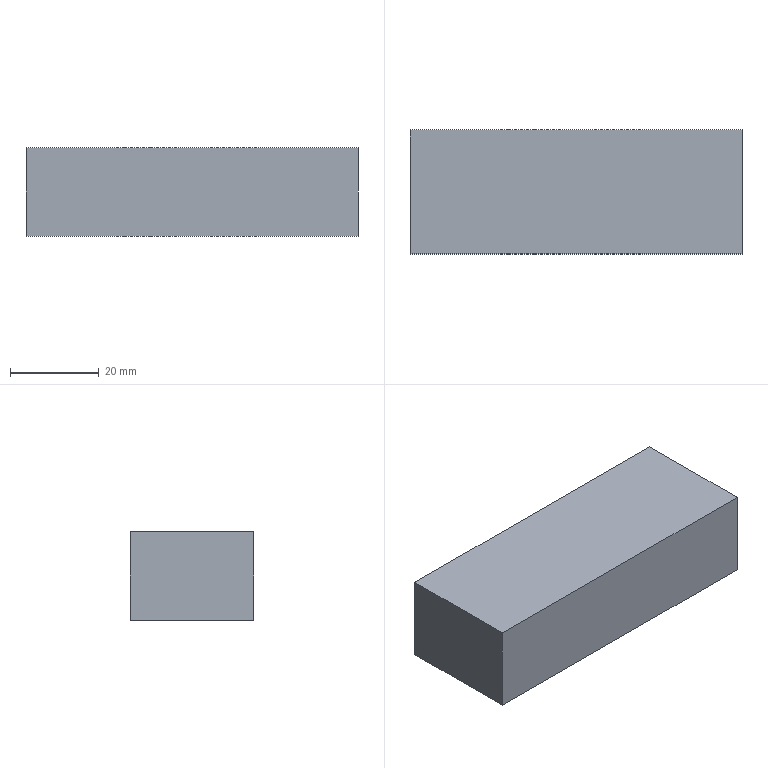Part | NX | features solid 2 | 1 solid | 6 faces | box 75 x 28 x 20 mm | volume 42000 mm3 | plane 6
STEP:
#1=CARTESIAN_POINT('',(-412.5,726.,-325.));
#2=VERTEX_POINT('',#1);
#3=CARTESIAN_POINT('',(-412.5,754.,-325.));
#4=VERTEX_POINT('',#3);
#5=CARTESIAN_POINT('',(-412.5,726.,-325.));
#6=DIRECTION('',(0.,1.,0.));
#7=VECTOR('',#6,1000.);
#8=LINE('',#5,#7);
#9=EDGE_CURVE('',#2,#4,#8,.T.);
#10=ORIENTED_EDGE('',*,*,#9,.F.);
#11=CARTESIAN_POINT('',(-412.5,726.,-305.));
#12=VERTEX_POINT('',#11);
#13=CARTESIAN_POINT('',(-412.5,726.,-305.));
#14=DIRECTION('',(0.,0.,-1.));
#15=VECTOR('',#14,1000.);
#16=LINE('',#13,#15);
#17=EDGE_CURVE('',#12,#2,#16,.T.);
#18=ORIENTED_EDGE('',*,*,#17,.F.);
#19=CARTESIAN_POINT('',(-412.5,754.,-305.));
#20=VERTEX_POINT('',#19);
#21=CARTESIAN_POINT('',(-412.5,726.,-305.));
#22=DIRECTION('',(0.,1.,0.));
#23=VECTOR('',#22,1000.);
#24=LINE('',#21,#23);
#25=EDGE_CURVE('',#12,#20,#24,.T.);
#26=ORIENTED_EDGE('',*,*,#25,.T.);
#27=CARTESIAN_POINT('',(-412.5,754.,-305.));
#28=DIRECTION('',(0.,0.,-1.));
#29=VECTOR('',#28,1000.);
#30=LINE('',#27,#29);
#31=EDGE_CURVE('',#20,#4,#30,.T.);
#32=ORIENTED_EDGE('',*,*,#31,.T.);
#33=EDGE_LOOP('',(#10,#18,#26,#32));
#34=FACE_BOUND('',#33,.T.);
#35=CARTESIAN_POINT('',(-412.5,726.,-305.));
#36=DIRECTION('',(-1.,0.,0.));
#37=DIRECTION('',(0.,0.,1.));
#38=AXIS2_PLACEMENT_3D('',#35,#36,#37);
#39=PLANE('',#38);
#40=ADVANCED_FACE('',(#34),#39,.T.);
#41=CARTESIAN_POINT('',(-337.5,754.,-325.));
#42=VERTEX_POINT('',#41);
#43=CARTESIAN_POINT('',(-412.5,754.,-325.));
#44=DIRECTION('',(1.,0.,0.));
#45=VECTOR('',#44,1000.);
#46=LINE('',#43,#45);
#47=EDGE_CURVE('',#4,#42,#46,.T.);
#48=ORIENTED_EDGE('',*,*,#47,.F.);
#49=ORIENTED_EDGE('',*,*,#31,.F.);
#50=CARTESIAN_POINT('',(-337.5,754.,-305.));
#51=VERTEX_POINT('',#50);
#52=CARTESIAN_POINT('',(-412.5,754.,-305.));
#53=DIRECTION('',(1.,0.,0.));
#54=VECTOR('',#53,1000.);
#55=LINE('',#52,#54);
#56=EDGE_CURVE('',#20,#51,#55,.T.);
#57=ORIENTED_EDGE('',*,*,#56,.T.);
#58=CARTESIAN_POINT('',(-337.5,754.,-305.));
#59=DIRECTION('',(0.,0.,-1.));
#60=VECTOR('',#59,1000.);
#61=LINE('',#58,#60);
#62=EDGE_CURVE('',#51,#42,#61,.T.);
#63=ORIENTED_EDGE('',*,*,#62,.T.);
#64=EDGE_LOOP('',(#48,#49,#57,#63));
#65=FACE_BOUND('',#64,.T.);
#66=CARTESIAN_POINT('',(-412.5,754.,-305.));
#67=DIRECTION('',(0.,1.,0.));
#68=DIRECTION('',(0.,0.,1.));
#69=AXIS2_PLACEMENT_3D('',#66,#67,#68);
#70=PLANE('',#69);
#71=ADVANCED_FACE('',(#65),#70,.T.);
#72=CARTESIAN_POINT('',(-337.5,726.,-325.));
#73=VERTEX_POINT('',#72);
#74=CARTESIAN_POINT('',(-337.5,764.,-325.));
#75=DIRECTION('',(0.,-1.,0.));
#76=VECTOR('',#75,1000.);
#77=LINE('',#74,#76);
#78=EDGE_CURVE('',#42,#73,#77,.T.);
#79=ORIENTED_EDGE('',*,*,#78,.F.);
#80=ORIENTED_EDGE('',*,*,#62,.F.);
#81=CARTESIAN_POINT('',(-337.5,726.,-305.));
#82=VERTEX_POINT('',#81);
#83=CARTESIAN_POINT('',(-337.5,764.,-305.));
#84=DIRECTION('',(0.,-1.,0.));
#85=VECTOR('',#84,1000.);
#86=LINE('',#83,#85);
#87=EDGE_CURVE('',#51,#82,#86,.T.);
#88=ORIENTED_EDGE('',*,*,#87,.T.);
#89=CARTESIAN_POINT('',(-337.5,726.,-305.));
#90=DIRECTION('',(0.,0.,-1.));
#91=VECTOR('',#90,1000.);
#92=LINE('',#89,#91);
#93=EDGE_CURVE('',#82,#73,#92,.T.);
#94=ORIENTED_EDGE('',*,*,#93,.T.);
#95=EDGE_LOOP('',(#79,#80,#88,#94));
#96=FACE_BOUND('',#95,.T.);
#97=CARTESIAN_POINT('',(-337.5,764.,-305.));
#98=DIRECTION('',(1.,0.,0.));
#99=DIRECTION('',(0.,1.,0.));
#100=AXIS2_PLACEMENT_3D('',#97,#98,#99);
#101=PLANE('',#100);
#102=ADVANCED_FACE('',(#96),#101,.T.);
#103=CARTESIAN_POINT('',(-337.5,726.,-325.));
#104=DIRECTION('',(-1.,0.,0.));
#105=VECTOR('',#104,1000.);
#106=LINE('',#103,#105);
#107=EDGE_CURVE('',#73,#2,#106,.T.);
#108=ORIENTED_EDGE('',*,*,#107,.F.);
#109=ORIENTED_EDGE('',*,*,#93,.F.);
#110=CARTESIAN_POINT('',(-337.5,726.,-305.));
#111=DIRECTION('',(-1.,0.,0.));
#112=VECTOR('',#111,1000.);
#113=LINE('',#110,#112);
#114=EDGE_CURVE('',#82,#12,#113,.T.);
#115=ORIENTED_EDGE('',*,*,#114,.T.);
#116=ORIENTED_EDGE('',*,*,#17,.T.);
#117=EDGE_LOOP('',(#108,#109,#115,#116));
#118=FACE_BOUND('',#117,.T.);
#119=CARTESIAN_POINT('',(-337.5,726.,-305.));
#120=DIRECTION('',(0.,-1.,0.));
#121=DIRECTION('',(0.,0.,-1.));
#122=AXIS2_PLACEMENT_3D('',#119,#120,#121);
#123=PLANE('',#122);
#124=ADVANCED_FACE('',(#118),#123,.T.);
#125=ORIENTED_EDGE('',*,*,#25,.F.);
#126=ORIENTED_EDGE('',*,*,#114,.F.);
#127=ORIENTED_EDGE('',*,*,#87,.F.);
#128=ORIENTED_EDGE('',*,*,#56,.F.);
#129=EDGE_LOOP('',(#125,#126,#127,#128));
#130=FACE_BOUND('',#129,.T.);
#131=CARTESIAN_POINT('',(-412.5,764.,-305.));
#132=DIRECTION('',(0.,0.,-1.));
#133=DIRECTION('',(-1.,0.,0.));
#134=AXIS2_PLACEMENT_3D('',#131,#132,#133);
#135=PLANE('',#134);
#136=ADVANCED_FACE('',(#130),#135,.F.);
#137=ORIENTED_EDGE('',*,*,#9,.T.);
#138=ORIENTED_EDGE('',*,*,#47,.T.);
#139=ORIENTED_EDGE('',*,*,#78,.T.);
#140=ORIENTED_EDGE('',*,*,#107,.T.);
#141=EDGE_LOOP('',(#137,#138,#139,#140));
#142=FACE_BOUND('',#141,.T.);
#143=CARTESIAN_POINT('',(-412.5,764.,-325.));
#144=DIRECTION('',(0.,0.,-1.));
#145=DIRECTION('',(-1.,0.,0.));
#146=AXIS2_PLACEMENT_3D('',#143,#144,#145);
#147=PLANE('',#146);
#148=ADVANCED_FACE('',(#142),#147,.T.);
#149=CLOSED_SHELL('',(#40,#71,#102,#124,#136,#148));
#150=MANIFOLD_SOLID_BREP('',#149);
#151=(LENGTH_UNIT()NAMED_UNIT(*)SI_UNIT(.MILLI.,.METRE.));
#152=UNCERTAINTY_MEASURE_WITH_UNIT(LENGTH_MEASURE(0.00001),#151,'','');
#153=(NAMED_UNIT(*)PLANE_ANGLE_UNIT()SI_UNIT($,.RADIAN.));
#154=(NAMED_UNIT(*)SI_UNIT($,.STERADIAN.)SOLID_ANGLE_UNIT());
#155=(GEOMETRIC_REPRESENTATION_CONTEXT(3)GLOBAL_UNCERTAINTY_ASSIGNED_CONTEXT((#152))GLOBAL_UNIT_ASSIGNED_CONTEXT((#151,#153,#154))REPRESENTATION_CONTEXT('',''));
#156=ADVANCED_BREP_SHAPE_REPRESENTATION('',(#150),#155);